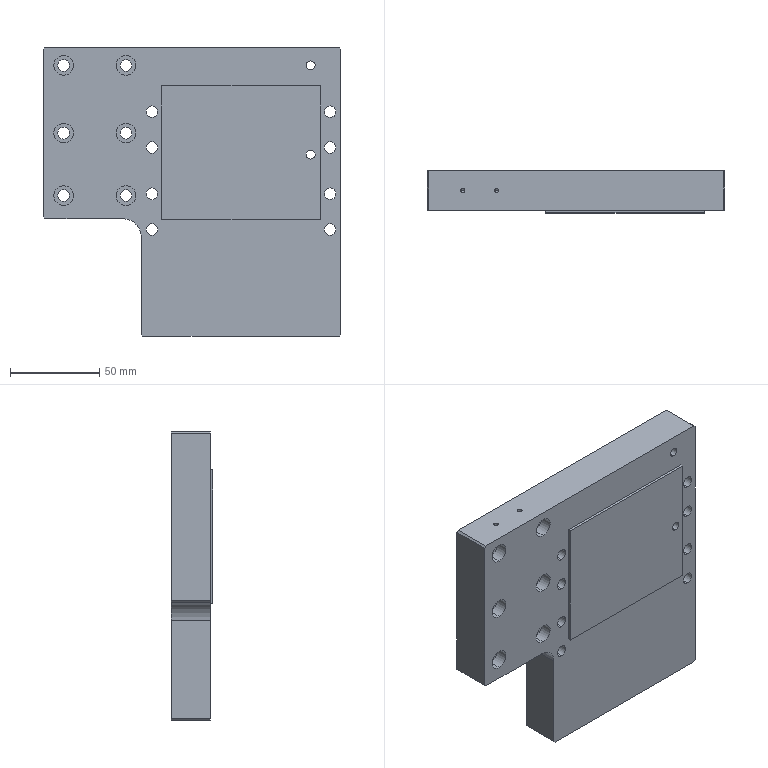Part | STEP file | 1 solid | 125 faces | box 167 x 23.5 x 162 mm | volume 506457 mm3 | cylinder 77 | plane 32 | cone 16 | commonest cylinder face diameters 11 x28 6.5 x16 3.3 x12 6.6 x12 2.5 x4 5 x4